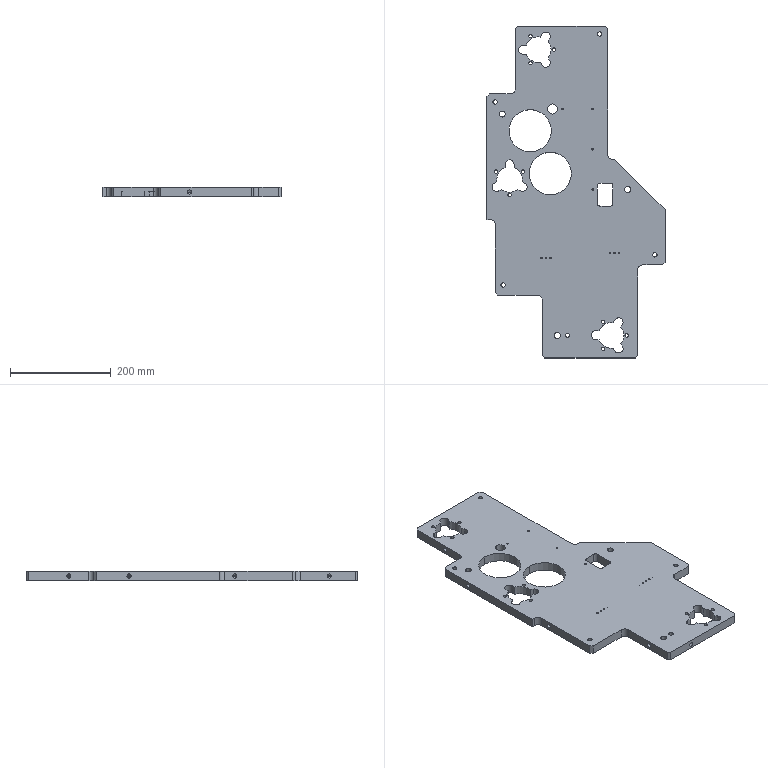NC program | NX | posted with a generic post | part box 354 x 660 x 18 mm
Whole program:
N10 G17 G21 G94 G90
(FACE_MILLING_COPY , TOOL : D8JING)
N12 T09 M6
N14 G54
N16 G17 G0 G90 X-330. Y-129.314 S6500 M3
N18 G43 Z30. H9
N20 Z3.
N22 G94 G1 Z0. F1250.
N24 Y-123.657
N26 Y67.657
N28 X-326.657 Y71.
N30 X-326.
N32 Y-127.
N34 X-322.
N36 Y71.
N38 X-318.
N40 Y-127.
N42 X-314.
N44 Y71.
N46 X-310.
N48 Y-127.
N50 X-306.
N52 Y71.
N54 X-302.
N56 Y-127.
N58 X-298.
N60 Y71.
N62 X-294.
N64 Y-127.
N66 X-290.
N68 Y71.
N70 X-286.
N72 Y-127.
N74 X-282.
N76 Y71.
N78 X-278.
N80 Y-127.
N82 X-274.
N84 Y71.
N86 X-270.
N88 Y-127.
N90 X-266.
N92 Y71.
N94 X-262.
N96 Y-127.
N98 X-258.
N100 Y71.
N102 X-254.
N104 Y-127.
N106 X-250.
N108 Y71.
N110 X-246.
N112 Y-127.
N114 X-242.
N116 Y71.
N118 X-238.
N120 Y-127.
N122 X-234.
N124 Y71.
N126 X-230.
N128 Y-127.
N130 X-226.
N132 Y71.
N134 X-222.
N136 Y-127.
N138 X-218.
N140 Y71.
N142 X-214. Y71.084
N144 Y-127.
N146 X-210.
N148 Y73.683
N150 X-209. Y157.157
N152 X-206. Y160.157
N154 Y-127.
N156 X-202.
N158 Y164.157
N160 X-201.657 Y164.5
N162 X-198.
N164 Y-127.
N166 X-194.
N168 Y164.5
N170 X-190.
N172 Y-127.
N174 X-186.
N176 Y164.5
N178 X-182.
N180 Y-127.
N182 X-178.
N184 Y164.5
N186 X-174.
N188 Y-127.
N190 X-170.
N192 Y164.5
N194 X-166.
N196 Y-127.
N198 X-162.
N200 Y164.5
N202 X-158.
N204 Y-127.
N206 X-154. Y-127.084
N208 Y164.5
N210 X-150.
N212 Y-129.683
N214 X-149. Y-173.657
N216 X-146. Y-176.657
N218 Y164.5
N220 X-142.
N222 Y-180.657
N224 X-141.657 Y-181.
N226 X-138.
N228 Y164.5
N230 X-134.
N232 Y-181.
N234 X-130.
N236 Y164.5
N238 X-126.
N240 Y-181.
N242 X-122.
N244 Y164.5
N246 X-118.
N248 Y-181.
N250 X-114.
N252 Y164.5
N254 X-110.
N256 Y-181.
N258 X-106.
N260 Y164.5
N262 X-102.
N264 Y-181.
N266 X-98.
N268 Y164.5
N270 X-94.
N272 Y-181.
N274 X-90.
N276 Y164.5
N278 X-86.
N280 Y-181.
N282 X-82.
N284 Y164.5
N286 X-78.
N288 Y-181.
N290 X-74.
N292 Y164.5
N294 X-70.
N296 Y-181.
N298 X-66.
N300 Y164.5
N302 X-62. Y165.304
N304 Y-181.
N306 X-58.
N308 Y181.
N310 X-54.
N312 Y-181.
N314 X-50.
N316 Y181.
N318 X-46.
N320 Y-181.
N322 X-42.
N324 Y181.
N326 X-38.
N328 Y-181.
N330 X-34.
N332 Y181.
N334 X-30.
N336 Y-177.657
N338 X-26. Y-173.657
N340 Y181.
N342 X-22.
N344 Y-169.657
N346 X-18. Y-165.657
N348 Y181.
N350 X-14.
N352 Y-161.657
N354 X-10. Y-157.657
N356 Y181.
N358 X-6.
N360 Y-153.657
N362 X-2. Y-149.657
N364 Y181.
N366 X2.
N368 Y-145.657
N370 X6. Y-141.657
N372 Y181.
N374 X10.
N376 Y-137.657
N378 X14. Y-133.657
N380 Y181.
N382 X18.
N384 Y-129.657
N386 X22. Y-125.657
N388 Y181.
N390 X26.
N392 Y-121.657
N394 X30. Y-117.657
N396 Y181.
N398 X34.
N400 Y-113.657
N402 X38. Y-109.657
N404 Y181.
N406 X42.
N408 Y-105.657
N410 X46. Y-101.657
N412 Y181.
N414 X50.
N416 Y-97.657
N418 X54. Y-93.657
N420 Y181.
N422 X58.
N424 Y-89.657
N426 X62. Y-85.657
N428 Y181.
N430 X66.
N432 Y-81.657
N434 X69. Y-78.657
N436 X70. Y-69.683
N438 Y181.
N440 X74.
N442 Y-67.084
N444 X78. Y-67.
N446 Y181.
N448 X82.
N450 Y-67.
N452 X86.
N454 Y181.
N456 X90.
N458 Y-67.
N460 X94.
N462 Y181.
N464 X98.
N466 Y-67.
N468 X102.
N470 Y181.
N472 X106.
N474 Y-67.
N476 X110.
N478 Y181.
N480 X114.
N482 Y-67.
N484 X118.
N486 Y181.
N488 X122.
N490 Y-67.
N492 X126.
N494 Y181.
N496 X130.
N498 Y-67.
N500 X134.
N502 Y181.
N504 X138.
N506 Y-67.
N508 X142.
N510 Y181.
N512 X146.
N514 Y-67.
N516 X150.
N518 Y181.
N520 X154.
N522 Y-67.
N524 X158.
N526 Y181.
N528 X162.
N530 Y-67.
N532 X166.
N534 Y181.
N536 X170.
N538 Y-67.
N540 X174.
N542 Y181.
N544 X178.
N546 Y-67.
N548 X182.
N550 Y181.
N552 X186.
N554 Y-67.
N556 X190.
N558 Y181.
N560 X191.657
N562 X194. Y178.657
N564 Y-67.
N566 X198.
N568 Y174.657
N570 X199. Y173.657
N572 X202. Y125.804
N574 Y-67.
N576 X206.
N578 Y125.
N580 X210.
N582 Y-67.
N584 X214.
N586 Y125.
N588 X218.
N590 Y-67.
N592 X222.
N594 Y125.
N596 X226.
N598 Y-67.
N600 X230.
N602 Y125.
N604 X234.
N606 Y-67.
N608 X238.
N610 Y125.
N612 X242.
N614 Y-67.
N616 X246.
N618 Y125.
N620 X250.
N622 Y-67.
N624 X254.
N626 Y125.
N628 X258.
N630 Y-67.
N632 X262.
N634 Y125.
N636 X266.
N638 Y-67.
N640 X270.
N642 Y125.
N644 X274.
N646 Y-67.
N648 X278.
N650 Y125.
N652 X282.
N654 Y-67.
N656 X286.
N658 Y125.
N660 X290.
N662 Y-67.
N664 X294.
N666 Y125.
N668 X298.
N670 Y-67.
N672 X302.
N674 Y125.
N676 X306.
N678 Y-67.
N680 X310.
N682 Y125.
N684 X314.
N686 Y-67.
N688 X318.
N690 Y125.
N692 X322.
N694 Y-67.
N696 X326.
N698 Y125.
N700 X326.657
N702 X330. Y121.657
N704 Y-63.657
N706 Y-69.314
N708 Z3.
N710 G0 Z30.
N712 M5
N714 M2